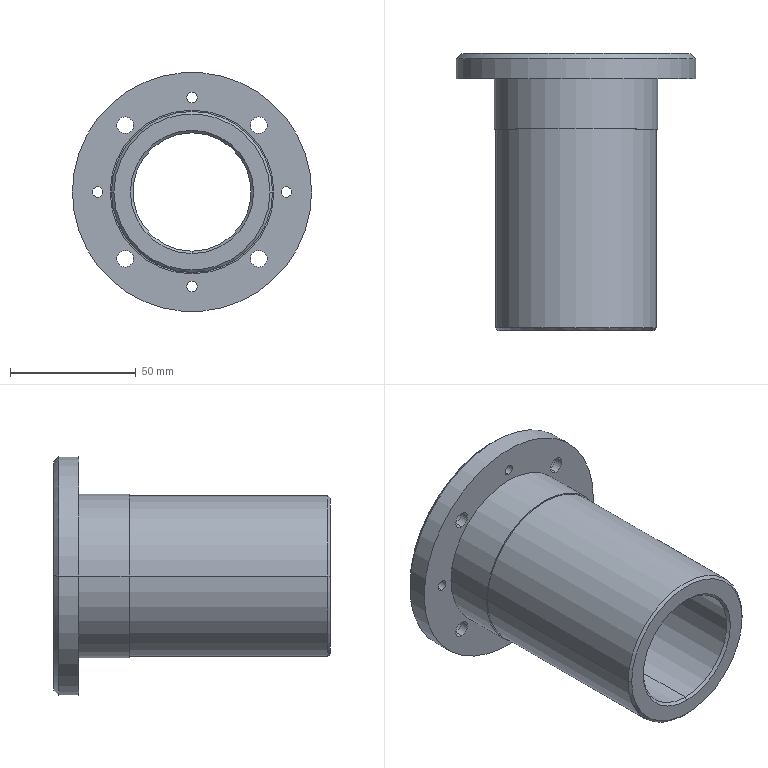Part | STEP file | 0229_211_Holder | 1 solid | 48 faces | box 95 x 110 x 95 mm | volume 199422 mm3 | cylinder 32 | cone 8 | plane 8 | commonest cylinder face diameters 4.2 x8 6.6 x8 11 x8 47 x2 64 x2 65 x2